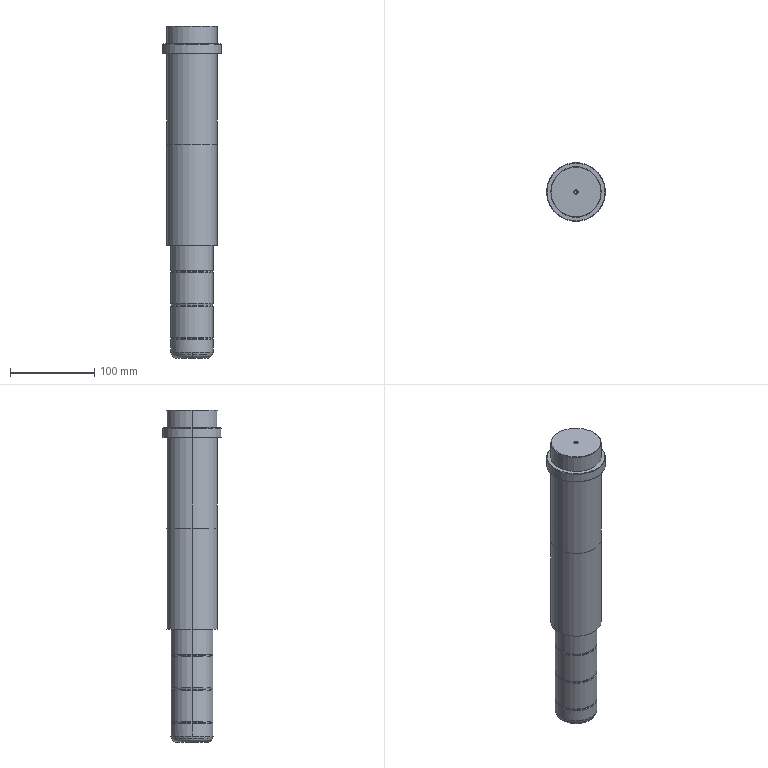Part | STEP file | Coluna superior CG - CG50196196 | 1 solid | 56 faces | box 70 x 70 x 395 mm | volume 1011106 mm3 | cylinder 20 | cone 16 | torus 14 | plane 6 | commonest cylinder face diameters 50 x8 4 x4 60 x4 59.98 x2 70 x2